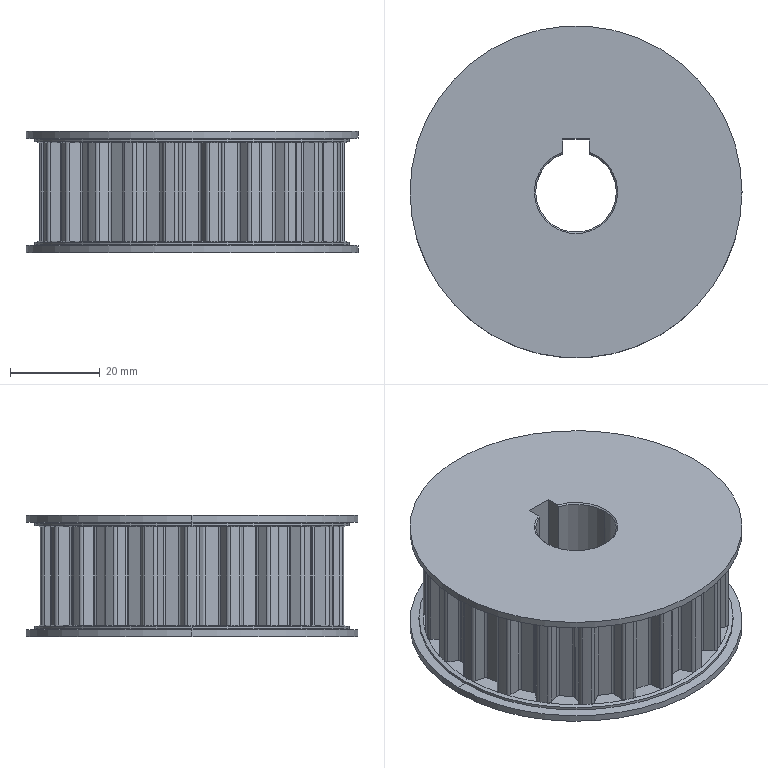Part | STEP file | Timing pulley 22-T10-φ18-27 | 1 solid | 283 faces | box 74 x 74 x 27 mm | volume 85142 mm3 | cylinder 150 | plane 119 | cone 14 | commonest cylinder face diameters 1.2 x56 1.6 x52 68.15 x23 3.3 x4 4.5 x4 70.03 x4